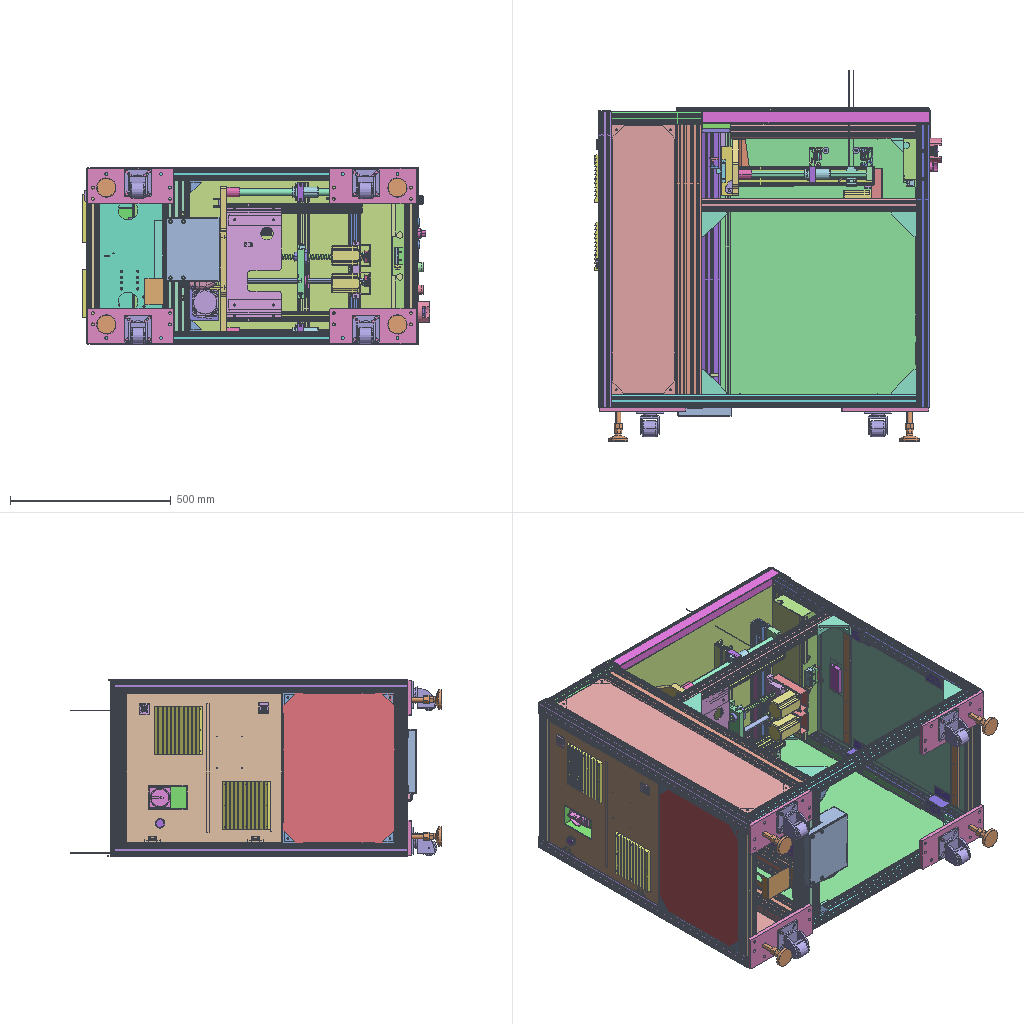Assembly | STEP file | 138 different items | 315 placed | box 1081 x 1155 x 550 mm
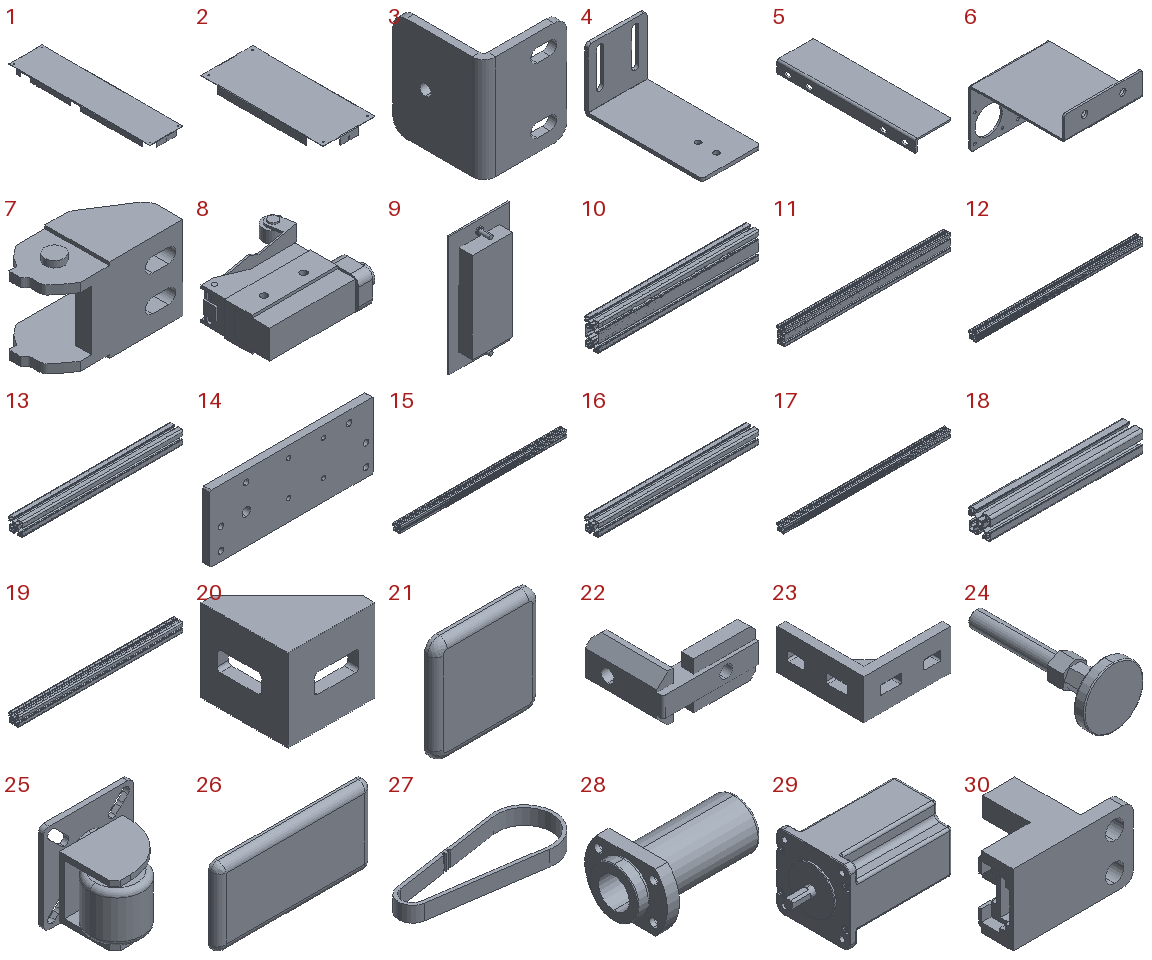Parts list (item | name | quantity | parent item | size | volume):
1 | - | x2 | - | 199 x 839 x 30 mm | 251918 mm3
2 | - | x1 | - | 199 x 469 x 30 mm | 138914 mm3
3 | - | x4 | - | 32 x 35 x 40 mm | 7142 mm3
4 | - | x1 | - | 35 x 70 x 37 mm | 6884 mm3
5 | - | x1 | - | 68 x 260 x 23 mm | 66736 mm3
6 | - | x1 | - | 82 x 100 x 83 mm | 26763 mm3
7 | Cable carrier connector 15x20B | x2 | - | 40 x 20 x 28 mm | 6776 mm3
8 | Limit switch D4MC-2000 | x1 | - | 71.855 x 71.5 x 21.7 mm | 42318 mm3
9 | Concealed handle XAD01_304_Yihe Da | x1 | - | 60 x 15 x 119 mm | 18675 mm3
10 | - | x2 | - | 470 x 40 x 80 mm | 377061 mm3
11 | - | x4 | - | 840 x 40 x 80 mm | 681890 mm3
12 | - | x2 | - | 880 x 40 x 40 mm | 420476 mm3
13 | - | x1 | - | 470 x 40 x 40 mm | 224394 mm3
14 | - | x4 | - | 270 x 12 x 110 mm | 348133 mm3
15 | MK-8-4040C-L-00 profile 4040C standard 950mm | x2 | - | 950 x 40 x 40 mm | 454336 mm3
16 | MK-8-4040C-L-00 profile 4040C standard 470mm | x3 | - | 470 x 40 x 40 mm | 224777 mm3
17 | MK-8-4040C-L-00 profile 4040C standard 920mm | x2 | - | 920 x 40 x 40 mm | 439989 mm3
18 | MK-8-4040C-L-00 profile 4040C standard 280mm | x2 | - | 280 x 40 x 40 mm | 133910 mm3
19 | MK-8-4040C-L-00 profile 4040C standard 670mm | x2 | - | 670 x 40 x 40 mm | 320427 mm3
20 | Die-cast aluminium connector, 40 series, 40mm face, standard type | x32 | - | 38 x 38 x 36 mm | 14409 mm3
21 | End cap panel MK-EC-B-4040x4.2 | x6 | - | 40 x 12.4 x 40 mm | 5038 mm3
22 | New in-slot right-angle connector, 40 series (with set screw) | x6 | - | 38 x 31 x 18.5 mm | 6406 mm3
23 | Die-cast aluminium connector, 40 series, 40mm face, reinforced type | x8 | - | 78 x 78 x 36 mm | 52626 mm3
24 | All-carbon-steel swivel leveling foot KCUF M16-100-60-electrophoretic black | x4 | - | 60 x 139 x 60 mm | 70730 mm3
25 | Medium 2-inch swivel caster J38NZN050R | x4 | - | 90 x 79 x 85 mm | 121466 mm3
26 | End cap panel MK-EC-B-3060x4 | x2 | - | 60 x 12.2 x 30 mm | 5483 mm3
27 | Timing belt 210-3M-9mm wide_16-36 | x2 | - | 90.97 x 35.218 x 9 mm | 3580 mm3
28 | Guided double-liner flanged linear bearing LML21-d20 | x2 | - | 80 x 54 x 38 mm | 45928 mm3
29 | Stepper motor SS2403A42A | x2 | - | 105.6 x 60 x 60 mm | 258866 mm3
30 | Photoelectric sensor PM-Y65 | x1 | - | 22.7 x 14.9 x 13.4 mm | 1660 mm3
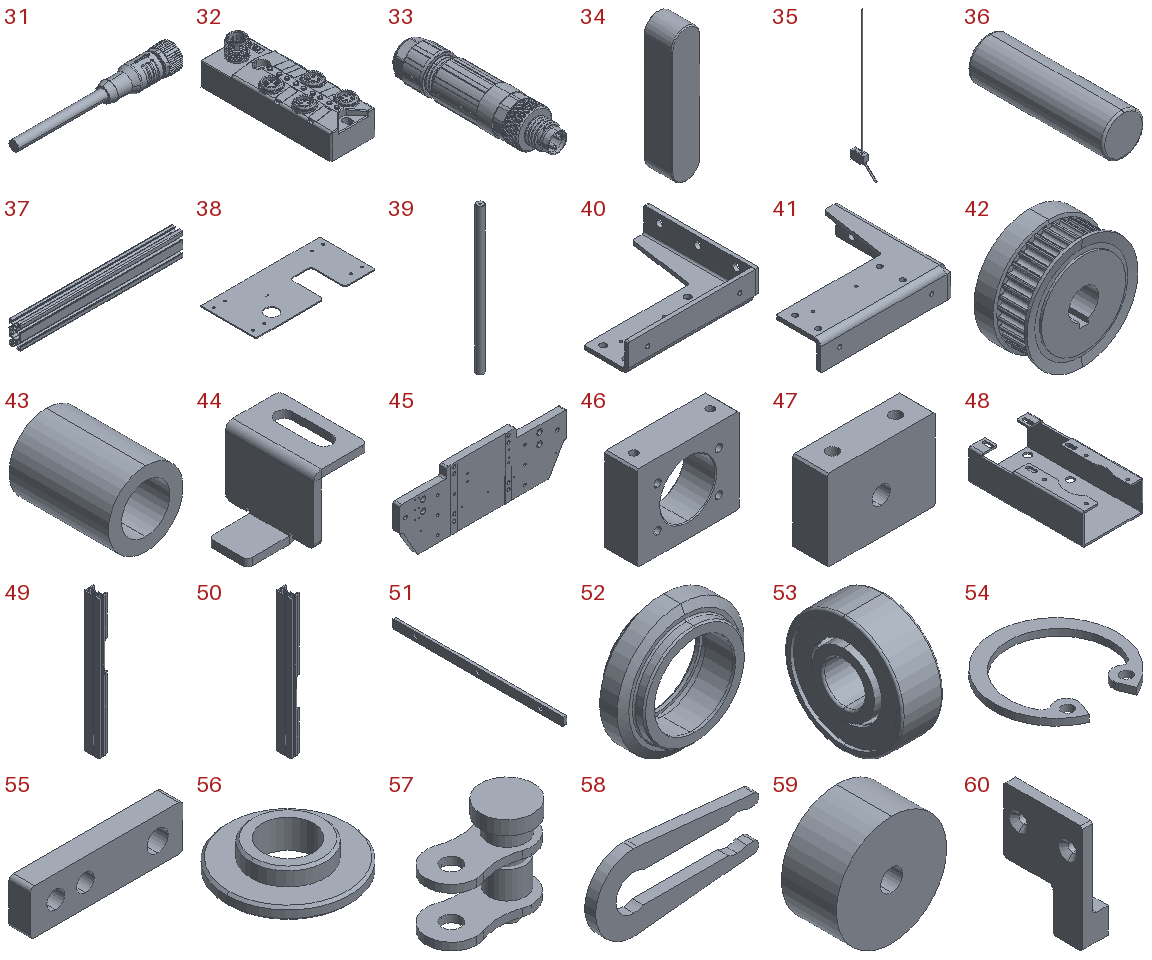31 | - | x1 | - | 99 x 14.979 x 14.996 mm | 5984 mm3
32 | I/O junction box 23N4S1 | x1 | - | 29.939 x 86.939 x 25.75 mm | 38975 mm3
33 | Plug (straight male) | x4 | - | - | -
34 | Type A plain key 3x3x14 | x2 | - | 3 x 3 x 14 mm | 119.894 mm3
35 | Miniature photoelectric sensor CX-442 | x2 | - | 11.2 x 58.715 x 345.215 mm | 7993 mm3
36 | - | x2 | - | 6 x 19.5 x 6 mm | 550.638 mm3
37 | - | x2 | - | 417 x 30 x 60.001 mm | 241330 mm3
38 | - | x1 | - | 365 x 170 x 3 mm | 161069 mm3
39 | - | x2 | - | 20 x 20 x 410 mm | 128595 mm3
40 | - | x1 | - | 170 x 145 x 37 mm | 104270 mm3
41 | - | x1 | - | 170 x 145 x 37 mm | 104662 mm3
42 | - | x2 | - | 37 x 19 x 37 mm | 15386 mm3
43 | - | x2 | - | 30 x 40 x 30 mm | 16328 mm3
44 | - | x1 | - | 19.5 x 18 x 15 mm | 668.205 mm3
45 | - | x1 | - | 482 x 20 x 176 mm | 1391575 mm3
46 | - | x2 | - | 60 x 19 x 50 mm | 36440 mm3
47 | - | x2 | - | 60 x 19 x 45 mm | 39956 mm3
48 | - | x2 | - | 68 x 128 x 35 mm | 37554 mm3
49 | - | x1 | - | 35 x 55 x 500 mm | 378713 mm3
50 | - | x1 | - | 35 x 55 x 500 mm | 378713 mm3
51 | - | x2 | - | 9 x 410 x 20.4 mm | 65356 mm3
52 | - | x4 | - | 25 x 8.5 x 25 mm | 1521 mm3
53 | PN_0001 Deep groove ball bearing 606-ZZ | x8 | - | 6 x 17 x 17 mm | 776.566 mm3
54 | PN_0001 Bore retaining ring type A 17 | x8 | - | 18.3 x 17.603 x 1 mm | 85.781 mm3
55 | - | x4 | - | 36 x 5 x 10.6 mm | 1667 mm3
56 | - | x4 | - | 15 x 15 x 3.5 mm | 281.21 mm3
57 | 06B side guide wheel chain | x2 | - | 18.325 x 9 x 17.4 mm | 854.513 mm3
58 | 06B side guide wheel chain link | x2 | - | 15 x 1 x 7 mm | 49.292 mm3
59 | - | x2 | - | 20 x 10 x 20 mm | 2790 mm3
60 | - | x1 | - | 13 x 40 x 55 mm | 9570 mm3
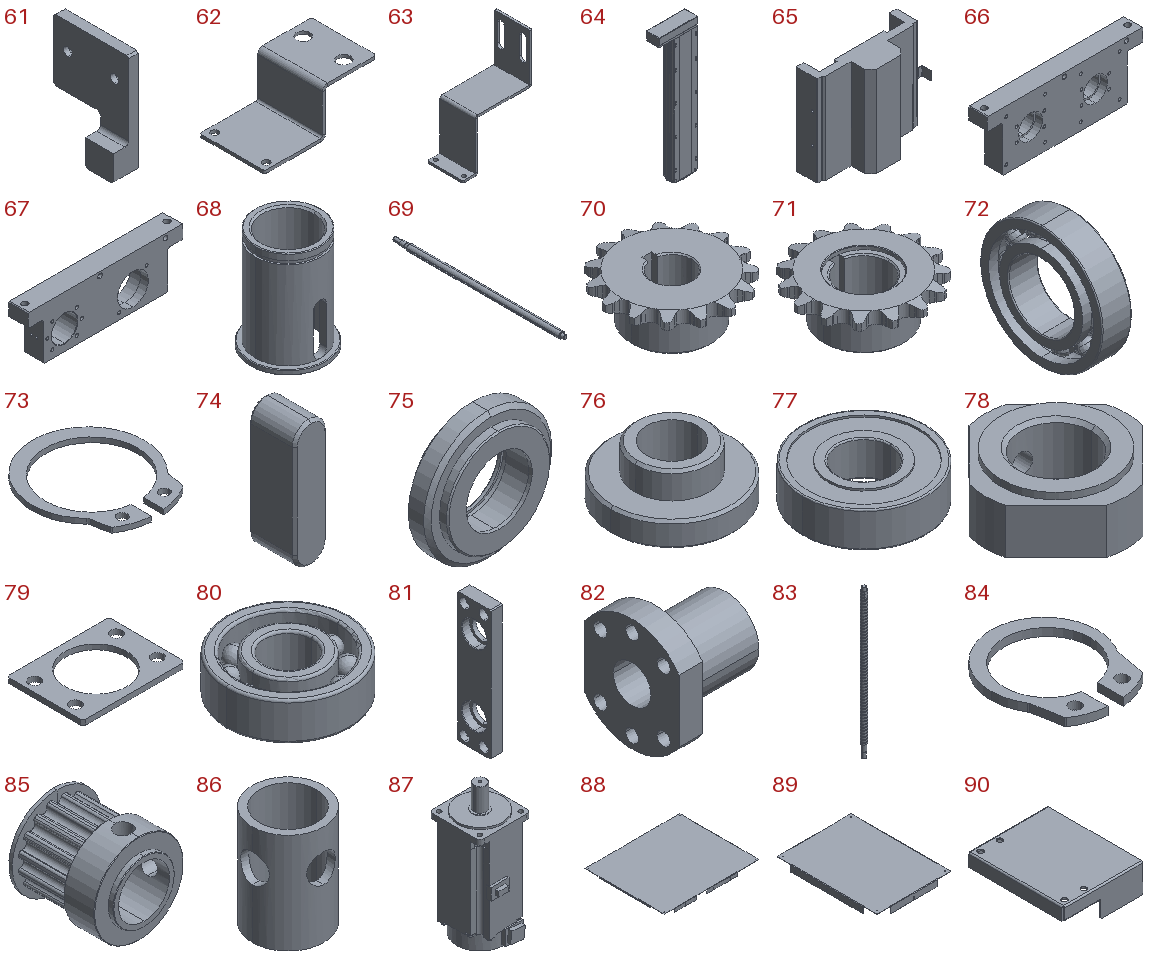61 | - | x1 | - | 13 x 40 x 55 mm | 9570 mm3
62 | - | x1 | - | 55 x 32 x 23.5 mm | 3494 mm3
63 | - | x1 | - | 62 x 32 x 90 mm | 8899 mm3
64 | Single-axis manipulator CFS17-L10-650-BR-T750-C4-MB-3M-body | x1 | - | 280.5 x 91 x 933.5 mm | 7444540 mm3
65 | Single-axis manipulator CFS17-L10-650-BR-T750-C4-MB-3M-slider | x1 | - | 177 x 71 x 152 mm | 741184 mm3
66 | - | x1 | - | 180 x 21 x 68 mm | 190682 mm3
67 | - | x1 | - | 170 x 21 x 57 mm | 135678 mm3
68 | - | x1 | - | 23 x 23 x 31.4 mm | 3535 mm3
69 | - | x1 | - | 16 x 443 x 16 mm | 80862 mm3
70 | - | x1 | - | 50.395 x 50.132 x 19 mm | 15455 mm3
71 | - | x1 | - | 50.395 x 50.132 x 19.5 mm | 13040 mm3
72 | Bearing 6904Z | x1 | - | 9 x 37 x 37 mm | 4601 mm3
73 | Shaft retaining ring type A 20 | x1 | - | 22.5 x 25.161 x 1 mm | 155.824 mm3
74 | - | x1 | - | 3.9 x 5.5 x 15 mm | 300.753 mm3
75 | - | x4 | - | 31 x 9 x 31 mm | 3611 mm3
76 | - | x4 | - | 15 x 15 x 6.2 mm | 541.108 mm3
77 | Bearing 6001ZZ | x2 | - | 28 x 28 x 8 mm | 3776 mm3
78 | - | x1 | - | 22 x 22 x 8 mm | 1773 mm3
79 | - | x2 | - | 40 x 30 x 2 mm | 1364 mm3
80 | Bearing 6000Z_P5_BONA_eco-friendly | x2 | - | 26 x 26 x 8 mm | 2544 mm3
81 | - | x1 | - | 12 x 35 x 135 mm | 43258 mm3
82 | Nut SFU01604-4 | x1 | in Ball screw assembly SFUR01604T4DFC7-445-P0 | 40 x 40 x 48 mm | 25660 mm3
83 | Ball screw assembly SFUR1604-445 | x1 | in Ball screw assembly SFUR01604T4DFC7-445-P0 | 16 x 16 x 445 mm | 80049 mm3
84 | Shaft retaining ring type A 12 | x1 | - | 13.6 x 15.973 x 1 mm | 68.14 mm3
85 | - | x2 | - | 17.5 x 18 x 17.5 mm | 1873 mm3
86 | - | x2 | - | 10 x 10 x 14 mm | 370.028 mm3
87 | Servo motor HG-KN73BJK-S100 750w_with brake_with keyway_Mitsubishi | x1 | - | 80.44 x 89.02 x 202.7 mm | 918886 mm3
88 | - | x1 | - | 798 x 668 x 30 mm | 686782 mm3
89 | - | x1 | - | 349 x 469 x 30 mm | 233516 mm3
90 | - | x1 | - | 166 x 200 x 60 mm | 160354 mm3
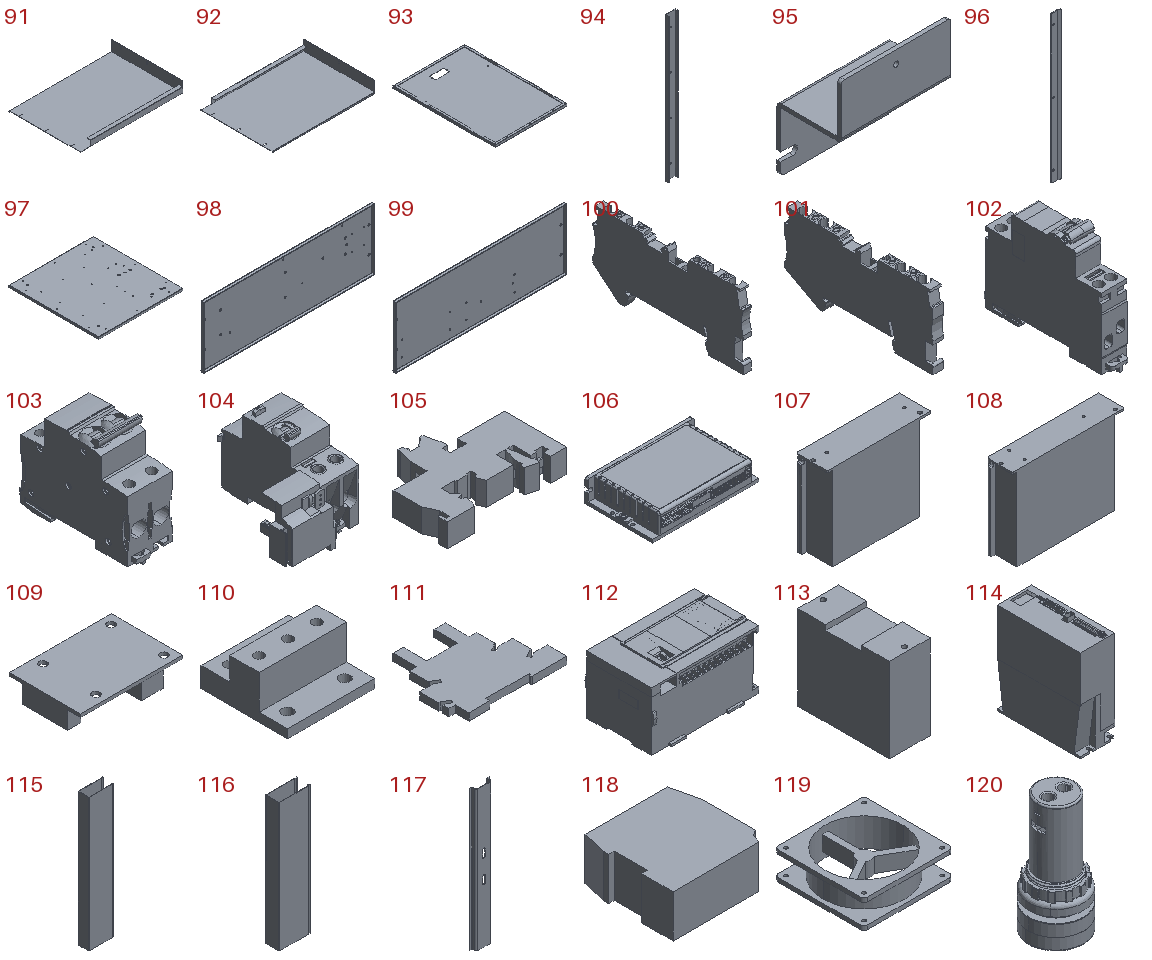91 | - | x1 | - | 790 x 550 x 88 mm | 1058095 mm3
92 | - | x1 | - | 790 x 550 x 88 mm | 1059109 mm3
93 | - | x1 | - | 467 x 667 x 16 mm | 433959 mm3
94 | - | x2 | - | 30 x 10 x 440 mm | 30430 mm3
95 | - | x4 | - | 70 x 41 x 71.5 mm | 18730 mm3
96 | - | x1 | - | 22.338 x 5 x 350 mm | 15718 mm3
97 | - | x1 | - | 400 x 425 x 10 mm | 275109 mm3
98 | - | x1 | - | 398 x 7.5 x 143 mm | 93935 mm3
99 | - | x1 | - | 398 x 7.5 x 143 mm | 94056 mm3
100 | Feed-through terminal block PT 1.5-S-QUATTRO | x27 | - | 3.5 x 63.2 x 30.5 mm | 4808 mm3
101 | Feed-through terminal block PT2,5-QUATTRO-3209578 | x6 | - | 5.15 x 72.2 x 35.25 mm | 9561 mm3
102 | Schneider miniature circuit breaker iDPNN-1P+N-C10A | x1 | - | 17.5 x 90.6 x 73.848 mm | 76092 mm3
103 | Miniature circuit breaker IC65N-2P-C16A | x1 | - | 35.4 x 93.9 x 74.3 mm | 159125 mm3
104 | Residual current device Vigi-iC65-ELE-2P-40A-30mA-A | x1 | - | 76.2 x 105.618 x 73.908 mm | 172404 mm3
105 | End bracket-E UK-1201442 | x4 | - | 50.5 x 35.3 x 9.5 mm | 9735 mm3
106 | Stepper motor driver DM542-KK V3.0 | x2 | - | 119 x 77.6 x 25.5 mm | 99944 mm3
107 | Switching power supply LRS-50-24 (Mean Well) | x1 | - | 99 x 30 x 82 mm | 213867 mm3
108 | Switching power supply LRS-100-48 | x1 | - | 129 x 30 x 97 mm | 340596 mm3
109 | PCB assembly | x1 | - | 54 x 38 x 11.5 mm | 8666 mm3
110 | Six-position earth copper block | x2 | - | 30.3 x 30.2 x 15 mm | 7115 mm3
111 | Ultra-miniature medium-power relay HF41F_24-ZST and socket 41F-1Z-C2-1 | x1 | - | 88 x 75.5 x 6.1 mm | 25363 mm3
112 | PLC module FX5U-32MT_ES | x1 | - | 150 x 96.4 x 84.9 mm | 980252 mm3
113 | PLC expansion IO FX5-16ET_ES8 (inputs, 8 outputs, transistor sink type) | x1 | - | 40 x 90 x 83 mm | 291482 mm3
114 | Servo drive MR-JE-70A | x1 | - | 70 x 168 x 191.95 mm | 896378 mm3
115 | Cable trough 35_L430 | x2 | - | 80.625 x 35 x 430 mm | 84214 mm3
116 | Cable trough 35_L330 | x3 | - | 80.625 x 35 x 330 mm | 64629 mm3
117 | Guide rail L_L245 | x2 | - | 35 x 8.3 x 245 mm | 11487 mm3
118 | EMC filter FIL-1S-1-10A-230AC-UT   1292320 | x1 | - | 99.5 x 99 x 45 mm | 422145 mm3
119 | Axial fan 1238A2MBL | x1 | - | 120 x 120 x 38 mm | 111801 mm3
120 | Indicator light AD17-22-AC220VW white | x1 | - | 29 x 29.009 x 63.018 mm | 9405 mm3
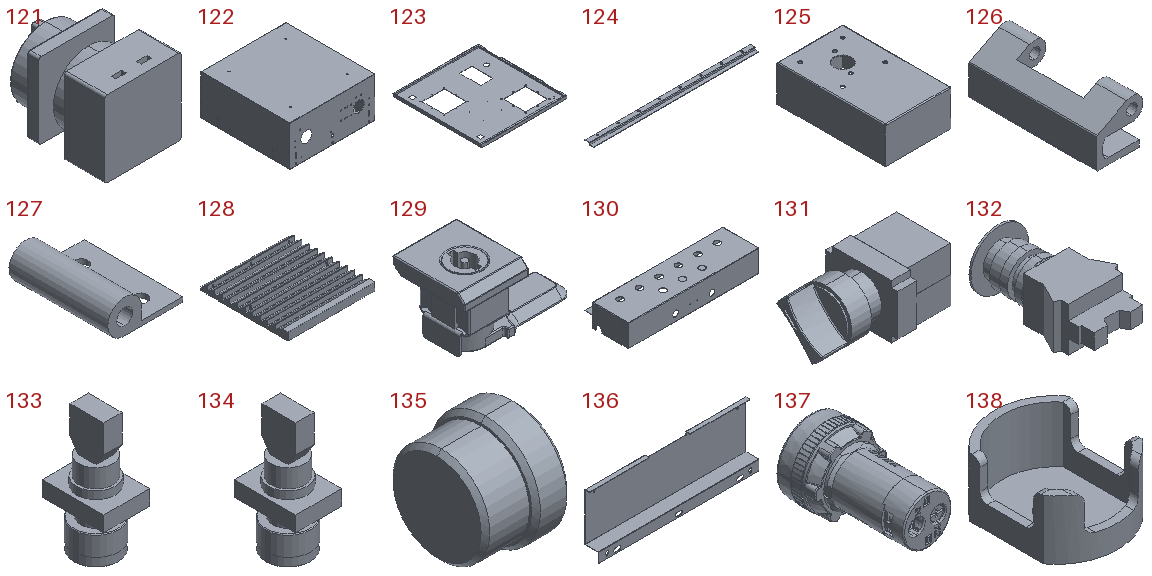121 | Power switch LW42B2-1824_L | x1 | - | 65.5 x 92 x 65.5 mm | 250369 mm3
122 | - | x1 | - | 465 x 486 x 234 mm | 846762 mm3
123 | - | x1 | - | 465 x 484 x 17 mm | 267277 mm3
124 | - | x1 | - | 400 x 21 x 6 mm | 10098 mm3
125 | - | x1 | - | 74 x 122 x 41 mm | 24069 mm3
126 | Hinge CL237Z3H001-01 | x2 | in Hinge CL237Z3H001 | 17.5 x 48 x 18 mm | 5234 mm3
127 | Hinge CL237Z3H001-02 | x2 | in Hinge CL237Z3H001 | 19 x 25 x 8.5 mm | 1495 mm3
128 | Class B ventilation filter assembly ZL-803 (7032 adhesive) | x2 | - | 150 x 150 x 28 mm | 421271 mm3
129 | Cylinder lock MS813-Shengjiu | x2 | - | 58.793 x 35 x 31.6 mm | 16415 mm3
130 | - | x1 | - | 469 x 158.8 x 80 mm | 180608 mm3
131 | Short-handle selector switch XB2-BD21C | x1 | - | 70 x 40 x 30 mm | 44517 mm3
132 | - | x1 | - | 44.567 x 87.5 x 40 mm | 63672 mm3
133 | Green illuminated pushbutton XB2-BW33B1C with 1 NO contact | x1 | - | 30 x 40 x 80 mm | 40739 mm3
134 | Blue illuminated pushbutton XB2-BW36B1C with 1 NO contact | x1 | - | 30 x 40 x 80 mm | 40739 mm3
135 | Panel plug T02 | x2 | - | 18 x 25 x 25 mm | 7618 mm3
136 | - | x1 | - | 470 x 39.5 x 167.8 mm | 118270 mm3
137 | Buzzer XB2BSB4LC | x1 | - | 29.699 x 50.596 x 29.699 mm | 12548 mm3
138 | - | x1 | - | 64 x 80 x 38.5 mm | 37425 mm3
Placements (level | parent | child | x y z in mm | rotation matrix by rows), first 274 of 336 lines:
1 | subassembly 2 | subassembly 3 | 777.434 1281.272 1459.066 | -1 0 0 0 1 0 0 0 -1
1 | subassembly 2 | subassembly 3 | 777.434 1281.272 2007.466 | 1 0 0 0 1 0 0 0 1
1 | subassembly 2 | subassembly 4 | 777.434 1740.472 1733.266 | 1 0 0 0 0 1 0 -1 0
1 | subassembly 2 | subassembly 5 | 677.434 1605.272 1965.766 | 0 1 0 0 0 1 1 0 -0
1 | subassembly 2 | subassembly 5 | 677.434 1605.272 1500.766 | 0 1 0 0 0 -1 -1 0 0
1 | subassembly 2 | subassembly 6 | 922.434 1263.772 1878.266 | 0 0 1 -1 0 0 0 -1 0
1 | subassembly 2 | subassembly 7 | 914.434 1189.272 1583.266 | -1 0 0 0 0 1 0 1 -0
1 | subassembly 2 | subassembly 5 | 677.434 1305.272 1965.766 | 0 1 0 0 0 1 1 0 -0
1 | subassembly 2 | subassembly 5 | 677.434 1305.272 1500.766 | 0 1 0 0 0 -1 -1 0 0
1 | subassembly 2 | subassembly 8 | 817.434 941.272 1623.266 | 0 -1 0 0 0 -1 1 0 -0
1 | subassembly 2 | Cable carrier connector 15x20B | 922.434 1230.772 1911.766 | 0 1 0 1 0 0 0 0 -1
1 | subassembly 2 | Cable carrier connector 15x20B | 1054.434 1486.772 1885.766 | 0 -1 0 1 0 0 0 0 1
1 | subassembly 2 | Limit switch D4MC-2000 | 1615.435 1519.422 1745.966 | 0 1 0 0 0 -1 -1 0 0
1 | subassembly 2 | Concealed handle XAD01_304_Yihe Da | 1654.034 1457.272 1733.266 | 0 1 0 -1 0 0 0 0 1
1 | subassembly 2 | subassembly 9 | 817.116 381.543 740.825 | 1 0 0 0 1 0 0 0 1
2 | subassembly 9 | subassembly 10 | 100.319 459.73 1227.441 | 0 0 1 0 1 0 -1 0 0
2 | subassembly 9 | subassembly 10 | 100.319 1339.73 757.441 | 0 0 1 0 -1 0 1 0 0
2 | subassembly 9 | subassembly 11 | 120.319 479.73 1062.441 | 0 -1 0 1 0 0 0 0 1
2 | subassembly 9 | subassembly 11 | 120.319 479.73 882.441 | 0 -1 0 1 0 0 0 0 1
2 | subassembly 9 | subassembly 11 | 100.319 479.73 737.441 | 0 0 1 1 0 0 0 1 -0
2 | subassembly 9 | subassembly 11 | 100.319 479.73 1247.441 | 0 0 1 1 0 0 0 1 -0
2 | subassembly 9 | subassembly 12 | 830.319 1319.73 1247.441 | 0 0 -1 -1 0 0 0 1 0
2 | subassembly 9 | subassembly 13 | 830.319 1299.73 757.441 | 0 0 -1 0 1 0 1 0 0
2 | subassembly 9 | subassembly 12 | 830.319 1319.73 737.441 | 0 0 1 -1 0 0 0 -1 0
2 | subassembly 9 | subassembly 14 | -177.681 433.73 719.441 | 1 0 0 0 -1 0 0 0 -1
2 | subassembly 9 | subassembly 14 | -177.681 433.73 1265.441 | 1 0 0 0 1 0 0 0 1
2 | subassembly 9 | subassembly 14 | 848.319 433.73 1265.441 | -1 0 0 0 -1 0 0 0 1
2 | subassembly 9 | subassembly 14 | 848.319 433.73 719.441 | -1 0 0 0 1 0 0 0 -1
2 | subassembly 9 | MK-8-4040C-L-00 profile 4040C standard 950mm | -139.681 459.73 737.441 | 1 0 0 0 1 0 0 0 1
2 | subassembly 9 | MK-8-4040C-L-00 profile 4040C standard 950mm | -139.681 459.73 1247.441 | 1 0 0 0 1 0 0 0 1
2 | subassembly 9 | MK-8-4040C-L-00 profile 4040C standard 470mm | -159.681 459.73 757.441 | 0 0 -1 0 1 0 1 0 0
2 | subassembly 9 | MK-8-4040C-L-00 profile 4040C standard 470mm | 830.319 459.73 757.441 | 0 0 -1 0 1 0 1 0 0
2 | subassembly 9 | MK-8-4040C-L-00 profile 4040C standard 470mm | -159.681 1339.73 757.441 | 0 0 -1 0 1 0 1 0 0
2 | subassembly 9 | MK-8-4040C-L-00 profile 4040C standard 920mm | -159.681 439.73 1247.441 | 0 -1 0 1 0 0 0 0 1
2 | subassembly 9 | MK-8-4040C-L-00 profile 4040C standard 920mm | -159.681 439.73 737.441 | 0 -1 0 1 0 0 0 0 1
2 | subassembly 9 | MK-8-4040C-L-00 profile 4040C standard 280mm | -139.681 1339.73 1247.441 | 1 0 0 0 1 0 0 0 1
2 | subassembly 9 | MK-8-4040C-L-00 profile 4040C standard 280mm | -139.681 1339.73 737.441 | 1 0 0 0 1 0 0 0 1
2 | subassembly 9 | MK-8-4040C-L-00 profile 4040C standard 670mm | 140.319 1299.73 737.441 | 1 0 0 0 1 0 0 0 1
2 | subassembly 9 | MK-8-4040C-L-00 profile 4040C standard 670mm | 140.319 1069.73 1247.441 | 1 0 0 0 1 0 0 0 1
2 | subassembly 9 | Die-cast aluminium connector, 40 series, 40mm face, standard type | -139.681 479.73 737.441 | 1 0 0 0 1 0 0 0 1
2 | subassembly 9 | Die-cast aluminium connector, 40 series, 40mm face, standard type | -139.681 1319.73 737.441 | 0 1 0 -1 0 0 0 0 1
2 | subassembly 9 | Die-cast aluminium connector, 40 series, 40mm face, standard type | 60.319 479.73 737.291 | 0 -1 0 1 0 0 0 0 1
2 | subassembly 9 | Die-cast aluminium connector, 40 series, 40mm face, standard type | 60.319 1319.73 737.441 | -1 0 0 0 -1 0 0 0 1
2 | subassembly 9 | Die-cast aluminium connector, 40 series, 40mm face, standard type | -139.681 1319.73 1247.441 | 1 0 0 0 -1 0 0 0 -1
2 | subassembly 9 | Die-cast aluminium connector, 40 series, 40mm face, standard type | -139.681 479.73 1247.441 | 0 1 0 1 0 0 0 0 -1
2 | subassembly 9 | Die-cast aluminium connector, 40 series, 40mm face, standard type | 60.319 479.73 1247.441 | -1 0 0 0 1 0 0 0 -1
2 | subassembly 9 | Die-cast aluminium connector, 40 series, 40mm face, standard type | 60.319 1319.73 1247.441 | 0 -1 0 -1 0 0 0 0 -1
2 | subassembly 9 | Die-cast aluminium connector, 40 series, 40mm face, standard type | 60.319 1339.73 1227.441 | -1 0 0 0 0 -1 0 -1 -0
2 | subassembly 9 | Die-cast aluminium connector, 40 series, 40mm face, standard type | 60.319 1339.73 757.441 | 0 -1 0 0 0 -1 1 0 -0
2 | subassembly 9 | Die-cast aluminium connector, 40 series, 40mm face, standard type | -139.681 1339.73 757.441 | 1 0 0 0 0 -1 0 1 0
2 | subassembly 9 | Die-cast aluminium connector, 40 series, 40mm face, standard type | 60.319 459.73 1227.441 | -1 0 0 0 0 -1 0 -1 -0
2 | subassembly 9 | Die-cast aluminium connector, 40 series, 40mm face, standard type | 60.319 459.73 757.441 | 0 -1 0 0 0 -1 1 0 0
2 | subassembly 9 | Die-cast aluminium connector, 40 series, 40mm face, standard type | 140.319 459.73 1227.441 | 0 1 0 0 0 -1 -1 0 0
2 | subassembly 9 | Die-cast aluminium connector, 40 series, 40mm face, standard type | 80.169 1319.73 1227.441 | 0 0 -1 0 -1 0 -1 0 0
2 | subassembly 9 | Die-cast aluminium connector, 40 series, 40mm face, standard type | 80.169 1319.73 757.441 | 0 0 -1 -1 0 0 0 1 -0
2 | subassembly 9 | Die-cast aluminium connector, 40 series, 40mm face, standard type | -139.681 1339.73 1227.441 | 0 1 0 0 0 -1 -1 0 0
2 | subassembly 9 | Die-cast aluminium connector, 40 series, 40mm face, standard type | 140.319 459.73 757.441 | 1 0 0 0 0 -1 0 1 0
2 | subassembly 9 | End cap panel MK-EC-B-4040x4.2 | -159.681 1363.93 737.441 | -1 0 0 0 -1 0 0 0 1
2 | subassembly 9 | End cap panel MK-EC-B-4040x4.2 | -159.681 1363.93 1247.441 | -1 0 0 0 -1 0 0 0 1
2 | subassembly 9 | New in-slot right-angle connector, 40 series (with set screw) | 834.319 1290.73 1238.341 | 0 0 -1 0 -1 0 -1 0 0
2 | subassembly 9 | New in-slot right-angle connector, 40 series (with set screw) | 826.319 1290.73 746.541 | 0 0 1 0 -1 0 1 0 -0
2 | subassembly 9 | Die-cast aluminium connector, 40 series, 40mm face, standard type | 122.319 479.73 1227.441 | 0 0 -1 1 0 0 0 -1 0
2 | subassembly 9 | Die-cast aluminium connector, 40 series, 40mm face, standard type | 78.319 479.73 1227.441 | 0 0 -1 1 0 0 0 -1 0
2 | subassembly 9 | Die-cast aluminium connector, 40 series, 40mm face, standard type | 122.319 1319.73 1227.441 | 0 0 -1 0 -1 0 -1 0 0
2 | subassembly 9 | Die-cast aluminium connector, 40 series, 40mm face, standard type | 122.319 1319.73 757.441 | 0 0 -1 -1 0 0 0 1 -0
2 | subassembly 9 | Die-cast aluminium connector, 40 series, 40mm face, standard type | 100.319 479.73 860.441 | -1 0 0 0 1 0 0 0 -1
2 | subassembly 9 | Die-cast aluminium connector, 40 series, 40mm face, standard type | 100.319 479.73 1084.441 | -1 0 0 0 1 0 0 0 -1
2 | subassembly 9 | Die-cast aluminium connector, 40 series, 40mm face, standard type | 100.319 1319.73 1084.441 | 0 -1 0 -1 0 0 0 0 -1
2 | subassembly 9 | Die-cast aluminium connector, 40 series, 40mm face, standard type | 100.319 1319.73 860.441 | 0 -1 0 -1 0 0 0 0 -1
2 | subassembly 9 | Die-cast aluminium connector, 40 series, 40mm face, standard type | -161.681 479.73 1227.441 | 0 0 -1 1 0 0 0 -1 0
2 | subassembly 9 | Die-cast aluminium connector, 40 series, 40mm face, standard type | -161.681 479.73 757.441 | 0 0 1 1 0 0 0 1 -0
2 | subassembly 9 | New in-slot right-angle connector, 40 series (with set screw) | 826.419 465.73 1241.441 | 0 0 1 0 1 0 -1 0 -0
2 | subassembly 9 | New in-slot right-angle connector, 40 series (with set screw) | 834.219 465.73 743.441 | 0 0 -1 0 1 0 1 0 0
2 | subassembly 9 | New in-slot right-angle connector, 40 series (with set screw) | -155.781 1333.73 743.441 | 0 0 -1 -1 0 0 0 1 0
2 | subassembly 9 | New in-slot right-angle connector, 40 series (with set screw) | -163.581 1333.73 1241.441 | 0 0 1 -1 0 0 0 -1 -0
2 | subassembly 9 | Die-cast aluminium connector, 40 series, 40mm face, standard type | -161.681 829.73 757.441 | 0 0 -1 -1 0 0 0 1 -0
2 | subassembly 9 | Die-cast aluminium connector, 40 series, 40mm face, standard type | -161.681 829.73 1227.441 | 0 0 1 -1 0 0 0 -1 -0
2 | subassembly 9 | Die-cast aluminium connector, 40 series, 40mm face, reinforced type | 140.319 479.73 719.441 | 1 0 0 0 1 0 0 0 1
2 | subassembly 9 | Die-cast aluminium connector, 40 series, 40mm face, reinforced type | 140.319 479.73 1265.441 | 0 1 0 1 0 0 0 0 -1
2 | subassembly 9 | Die-cast aluminium connector, 40 series, 40mm face, reinforced type | 140.319 1049.73 1265.441 | 1 0 0 0 -1 0 0 0 -1
2 | subassembly 9 | Die-cast aluminium connector, 40 series, 40mm face, reinforced type | 140.319 1279.73 719.441 | 0 1 0 -1 0 0 0 0 1
2 | subassembly 9 | Die-cast aluminium connector, 40 series, 40mm face, reinforced type | 810.319 479.73 1265.441 | -1 0 0 0 1 0 0 0 -1
2 | subassembly 9 | Die-cast aluminium connector, 40 series, 40mm face, reinforced type | 810.319 479.73 719.441 | 0 -1 0 1 0 0 0 0 1
2 | subassembly 9 | Die-cast aluminium connector, 40 series, 40mm face, reinforced type | 810.319 1279.73 719.441 | -1 0 0 0 -1 0 0 0 1
2 | subassembly 9 | Die-cast aluminium connector, 40 series, 40mm face, reinforced type | 810.319 1049.73 1265.441 | 0 -1 0 -1 0 0 0 0 -1
2 | subassembly 9 | End cap panel MK-EC-B-4040x4.2 | 830.319 1323.93 1247.441 | -1 0 0 0 -1 0 0 0 1
2 | subassembly 9 | End cap panel MK-EC-B-4040x4.2 | 830.319 1323.93 737.441 | -1 0 0 0 -1 0 0 0 1
2 | subassembly 9 | End cap panel MK-EC-B-4040x4.2 | 144.519 1339.73 1247.441 | 0 -1 0 1 0 0 0 0 1
2 | subassembly 9 | End cap panel MK-EC-B-4040x4.2 | 144.519 1339.73 737.441 | 0 -1 0 1 0 0 0 0 1
2 | subassembly 9 | Die-cast aluminium connector, 40 series, 40mm face, standard type | 78.319 479.73 757.441 | 0 0 1 1 0 0 0 1 -0
2 | subassembly 9 | Die-cast aluminium connector, 40 series, 40mm face, standard type | 122.319 479.73 757.441 | 0 0 -1 0 1 0 1 0 -0
2 | subassembly 9 | All-carbon-steel swivel leveling foot KCUF M16-100-60-electrophoretic black | -117.681 334.73 1205.441 | 0.6837 0 -0.7298 0 1 0 0.7298 0 0.6837
2 | subassembly 9 | All-carbon-steel swivel leveling foot KCUF M16-100-60-electrophoretic black | -117.681 334.73 779.441 | 0.6837 0 -0.7298 0 1 0 0.7298 0 0.6837
2 | subassembly 9 | All-carbon-steel swivel leveling foot KCUF M16-100-60-electrophoretic black | 788.319 334.73 779.441 | 0.6837 0 -0.7298 0 1 0 0.7298 0 0.6837
2 | subassembly 9 | All-carbon-steel swivel leveling foot KCUF M16-100-60-electrophoretic black | 788.319 334.73 1205.441 | 0.6837 0 -0.7298 0 1 0 0.7298 0 0.6837
2 | subassembly 9 | Medium 2-inch swivel caster J38NZN050R | -20.104 422.73 1219.864 | 0 0 -1 0 1 0 1 0 0
2 | subassembly 9 | Medium 2-inch swivel caster J38NZN050R | 689.504 422.73 1218.627 | 0 0 -1 0 1 0 1 0 0
2 | subassembly 9 | Medium 2-inch swivel caster J38NZN050R | -18.866 422.73 766.256 | 0 0 -1 0 1 0 1 0 0
2 | subassembly 9 | Medium 2-inch swivel caster J38NZN050R | 689.504 422.73 766.256 | 0 0 -1 0 1 0 1 0 0
1 | subassembly 2 | subassembly 15 | 804.051 1822.324 1868.016 | 1 0 0 0 1 0 0 0 1
2 | subassembly 15 | End cap panel MK-EC-B-3060x4 | 691.383 -280.052 12.751 | 0 -1 0 1 0 0 0 0 1
2 | subassembly 15 | End cap panel MK-EC-B-3060x4 | 691.383 -280.052 -322.25 | 0 -1 0 1 0 0 0 0 1
2 | subassembly 15 | Timing belt 210-3M-9mm wide_16-36 | 695.883 -353.982 -219.179 | 0 0 1 0.9944 -0.1061 0 0.1061 0.9944 -0
2 | subassembly 15 | Timing belt 210-3M-9mm wide_16-36 | 695.883 -353.982 -133.32 | 0 0 1 0.9982 0.06018 0 -0.06018 0.9982 0
2 | subassembly 15 | Guided double-liner flanged linear bearing LML21-d20 | 474.761 -275.052 64.251 | 1 0 0 0 0 -1 0 1 -0
2 | subassembly 15 | Guided double-liner flanged linear bearing LML21-d20 | 474.761 -275.052 -373.75 | 1 0 0 0 0 1 0 -1 0
2 | subassembly 15 | Stepper motor SS2403A42A | 682.544 -353.982 -219.179 | -1 0 0 0 1 0 0 0 -1
2 | subassembly 15 | Stepper motor SS2403A42A | 682.544 -353.982 -133.32 | -1 0 0 0 1 0 0 0 -1
2 | subassembly 15 | Photoelectric sensor PM-Y65 | 338.383 -297.152 -102.749 | 1 0 0 0 1 0 0 0 1
2 | subassembly 15 | subassembly 16 | 339.983 -272.068 -60.213 | 0 0.3525 0.9358 0 -0.9358 0.3525 1 0 0
2 | subassembly 15 | I/O junction box 23N4S1 | 405.833 -272.053 -8.1 | 0.000231 -1 0 -1 -0.000231 0 0 0 -1
2 | subassembly 15 | Plug (straight male) | 381.885 -280.309 -35.099 | 0.3271 0 -0.945 0.945 0 0.3271 0 -1 -0
2 | subassembly 15 | Plug (straight male) | 403.885 -280.304 -35.099 | -0.6482 0 0.7615 -0.7615 0 -0.6482 0 -1 -0
2 | subassembly 15 | Plug (straight male) | 392.881 -263.806 -35.099 | -0.6482 0 0.7615 -0.7615 0 -0.6482 0 -1 -0
2 | subassembly 15 | Plug (straight male) | 370.881 -263.811 -35.099 | 0.2554 0 -0.9668 0.9668 0 0.2554 0 -1 -0
2 | subassembly 15 | Type A plain key 3x3x14 | 707.883 -289.544 -216.452 | 0 0 1 -0.9931 -0.1171 0 0.1171 -0.9931 0
2 | subassembly 15 | Type A plain key 3x3x14 | 707.383 -289.752 -137.25 | 0 0 1 0 1 0 -1 0 0
2 | subassembly 15 | Miniature photoelectric sensor CX-442 | 613.883 -251.552 44.151 | 0 1 0 0 0 1 1 0 0
2 | subassembly 15 | subassembly 17 | 252.633 -264.052 -232.75 | 0 1 0 0.1702 0 0.9854 0.9854 0 -0.1702
2 | subassembly 15 | subassembly 17 | 252.633 -264.052 -76.749 | 0 1 0 0.6769 0 -0.736 -0.736 0 -0.6769
2 | subassembly 15 | Miniature photoelectric sensor CX-442 | 626.883 -251.052 -399.849 | 0 -1 0 0 0 1 -1 0 0
2 | subassembly 15 | subassembly 18 | 270.383 -280.052 12.751 | 1 0 0 0 0 -1 0 1 -0
2 | subassembly 15 | subassembly 18 | 270.383 -280.052 -322.25 | 1 0 0 0 0 -1 0 1 -0
2 | subassembly 15 | subassembly 19 | 355.383 -310.052 -154.75 | 0 -1 0 0 0 1 -1 0 0
2 | subassembly 15 | subassembly 20 | 674.383 -275.052 64.251 | 0 0 -1 -0.3045 -0.9525 0 -0.9525 0.3045 -0
2 | subassembly 15 | subassembly 20 | 674.383 -275.052 -373.75 | 0 0 -1 -0.7619 0.6477 0 0.6477 0.7619 -0
2 | subassembly 15 | subassembly 21 | 305.383 -252.052 -7.25 | -1 0 0 0 1 0 0 0 -1
2 | subassembly 15 | subassembly 22 | 305.383 -252.052 -307.25 | -1 0 0 0 1 0 0 0 -1
2 | subassembly 15 | subassembly 23 | 704.883 -288.798 -137.25 | 0 1 0 0 0 1 1 0 0
2 | subassembly 15 | subassembly 24 | 310.383 -275.052 64.251 | 0 -1 0 -0.9986 0 0.05221 -0.05221 0 -0.9986
2 | subassembly 15 | subassembly 25 | 497.739 -292.552 -112.749 | 0 1 0 1 0 0 0 0 -1
2 | subassembly 15 | subassembly 24 | 310.383 -275.052 -373.75 | 0 -1 0 0.5126 0 0.8586 -0.8586 0 0.5126
2 | subassembly 15 | subassembly 23 | 704.883 -289.048 -212.25 | 0 1 0 -0.9931 0 0.1171 0.1171 0 0.9931
2 | subassembly 15 | subassembly 26 | 250.383 -252.552 -174.75 | 0 1 0 0 0 -1 -1 0 0
2 | subassembly 15 | subassembly 27 | 500.261 -275.052 64.251 | 0 1 0 0 0 1 1 0 0
2 | subassembly 15 | subassembly 28 | 675.883 -272.552 64.251 | 0 -1 0 0 0 1 -1 0 0
2 | subassembly 15 | subassembly 28 | 675.883 -272.552 -373.75 | 0 -1 0 0 0 1 -1 0 0
2 | subassembly 15 | subassembly 27 | 500.261 -275.052 -373.75 | 0 1 0 0 0 1 1 0 0
2 | subassembly 15 | subassembly 29 | 717.544 -320.052 -133.25 | 0 0 -1 0 1 0 1 0 -0
2 | subassembly 15 | subassembly 29 | 717.544 -320.052 -219.25 | 0 0 -1 0 1 0 1 0 -0
2 | subassembly 15 | subassembly 30 | 655.383 -219.467 -154.75 | 0 0 1 0 1 0 -1 0 0
3 | subassembly 30 | subassembly 31 | -0.0 -0.0 -0.0 | 0 0 1 0 1 0 -1 0 -0
3 | subassembly 30 | subassembly 32 | -0.0 0.0 -134.622 | 0 0 -1 0 1 0 1 0 0
3 | subassembly 30 | subassembly 33 | 34.294 1.115 -3.5 | 0 -1 0 0 0 -1 1 0 0
3 | subassembly 30 | subassembly 33 | 34.294 1.115 -131.122 | 0 1 0 0 0 -1 -1 0 0
3 | subassembly 30 | subassembly 34 | 200.813 21.773 -24.973 | 0.4736 0 0.8808 0.8808 0 -0.4736 0 1 -0
4 | subassembly 34 | subassembly 35 | -6.597 27.473 34.415 | 1 0 0 0 1 0 0 0 1
4 | subassembly 34 | PN_0001 Deep groove ball bearing 606-ZZ | -6.597 26.473 34.415 | 0 1 0 -1 0 0 0 0 1
4 | subassembly 34 | PN_0001 Bore retaining ring type A 17 | -6.597 30.023 34.415 | 1 0 0 0 0 -1 0 1 -0
3 | subassembly 30 | subassembly 34 | -216.546 34.279 -109.65 | -0.9409 0 -0.3388 0.3388 0 -0.9409 0 -1 -0
4 | subassembly 34 | subassembly 35 | -6.597 27.473 34.415 | 1 0 0 0 1 0 0 0 1
4 | subassembly 34 | PN_0001 Deep groove ball bearing 606-ZZ | -6.597 26.473 34.415 | 0 1 0 -1 0 0 0 0 1
4 | subassembly 34 | PN_0001 Bore retaining ring type A 17 | -6.597 30.023 34.415 | 1 0 0 0 0 -1 0 1 -0
3 | subassembly 30 | subassembly 34 | 189.699 13.249 -109.65 | -0.5543 0 0.8323 -0.8323 0 -0.5543 0 -1 0
4 | subassembly 34 | subassembly 35 | -6.597 27.473 34.415 | 1 0 0 0 1 0 0 0 1
4 | subassembly 34 | PN_0001 Deep groove ball bearing 606-ZZ | -6.597 26.473 34.415 | 0 1 0 -1 0 0 0 0 1
4 | subassembly 34 | PN_0001 Bore retaining ring type A 17 | -6.597 30.023 34.415 | 1 0 0 0 0 -1 0 1 -0
3 | subassembly 30 | subassembly 34 | -198.44 18.483 -24.973 | 0.6862 0 -0.7274 -0.7274 0 -0.6862 0 1 0
4 | subassembly 34 | subassembly 35 | -6.597 27.473 34.415 | 1 0 0 0 1 0 0 0 1
4 | subassembly 34 | PN_0001 Deep groove ball bearing 606-ZZ | -6.597 26.473 34.415 | 0 1 0 -1 0 0 0 0 1
4 | subassembly 34 | PN_0001 Bore retaining ring type A 17 | -6.597 30.023 34.415 | 1 0 0 0 0 -1 0 1 -0
3 | subassembly 30 | subassembly 36 | -216.0 -0.335 15.5 | -1 0 0 0 0 1 0 1 0
3 | subassembly 30 | subassembly 36 | -210.0 -0.335 -145.122 | -1 0 0 0 0 1 0 1 -0
3 | subassembly 30 | subassembly 36 | 216.0 -0.335 15.5 | 1 0 0 0 0 -1 0 1 0
3 | subassembly 30 | subassembly 36 | 210.0 -0.335 -145.122 | 1 0 0 0 0 -1 0 1 0
3 | subassembly 30 | subassembly 37 | -228.0 -0.335 8.0 | -0.2046 -0.9788 0 -0.9788 0.2046 0 0 0 -1
3 | subassembly 30 | subassembly 37 | -222.0 -0.335 -142.622 | 0.564 -0.8258 0 0.8258 0.564 0 0 0 1
3 | subassembly 30 | subassembly 37 | 222.0 -0.335 -142.622 | 0.564 -0.8258 0 0.8258 0.564 0 0 0 1
3 | subassembly 30 | subassembly 37 | 228.0 -0.335 8.0 | -0.2046 -0.9788 0 -0.9788 0.2046 0 0 0 -1
3 | subassembly 30 | 06B side guide wheel chain | 81.359 15.415 -7.44 | -1 0 0 0 1 0 0 0 -1
3 | subassembly 30 | 06B side guide wheel chain link | 84.045 19.348 -3.44 | 0.564 0 0.8258 0.8258 0 -0.564 0 1 0
3 | subassembly 30 | 06B side guide wheel chain link | -185.568 14.417 -132.182 | 0.1764 0 0.9843 0.9843 0 -0.1764 0 1 -0
3 | subassembly 30 | 06B side guide wheel chain | -194.298 15.065 -127.182 | -0.8284 -0.5602 0 0.5602 -0.8284 0 0 0 1
3 | subassembly 30 | subassembly 38 | 235.0 19.915 -19.9 | 0 -1 0 0.766 0 -0.6428 0.6428 0 0.766
3 | subassembly 30 | subassembly 38 | 235.0 19.915 -114.722 | 0 -1 0 -0.9385 0 0.3454 -0.3454 0 -0.9385
3 | subassembly 30 | subassembly 39 | 230.0 29.415 -138.722 | 0 -1 0 -1 0 0 0 0 -1
3 | subassembly 30 | subassembly 40 | 230.0 24.415 4.1 | 0 -1 0 1 0 0 0 0 1
2 | subassembly 15 | subassembly 41 | 636.383 -280.552 51.251 | 0 -1 0 -1 0 0 0 0 -1
2 | subassembly 15 | subassembly 42 | 604.383 -263.052 -394.25 | 0 1 0 -1 0 0 0 0 1
2 | subassembly 15 | subassembly 43 | -309.473 -1236.771 -579.385 | 0 1 0 0 0 1 1 0 -0
3 | subassembly 43 | Single-axis manipulator CFS17-L10-650-BR-T750-C4-MB-3M-body | 424.636 462.856 228.719 | 1 0 0 0 1 0 0 0 1
3 | subassembly 43 | Single-axis manipulator CFS17-L10-650-BR-T750-C4-MB-3M-slider | 424.636 462.856 203.719 | 1 0 0 0 1 0 0 0 1
2 | subassembly 15 | subassembly 44 | 682.544 -250.052 -921.269 | 0 0 1 0 1 0 -1 0 0
3 | subassembly 44 | subassembly 45 | -744.019 -34.0 -10.5 | 1 0 0 0 0 1 0 -1 -0
3 | subassembly 44 | subassembly 46 | -739.019 -28.5 -182.283 | 1 0 0 0 0 1 0 -1 0
3 | subassembly 44 | subassembly 47 | -709.019 -35.0 -160.783 | -0.1171 -0.9931 0 -0.9931 0.1171 0 0 0 -1
3 | subassembly 44 | subassembly 48 | -709.019 -35.0 -190.5 | -0.9931 0 0.1171 0.1171 0 0.9931 0 1 0
3 | subassembly 44 | subassembly 49 | -709.019 -35.0 -29.5 | -0.9064 0.4223 0 -0.4223 -0.9064 0 0 0 1
3 | subassembly 44 | subassembly 50 | -709.019 -35.0 -163.283 | 0.9416 -0.3366 0 0.3366 0.9416 0 0 0 1
3 | subassembly 44 | Bearing 6904Z | -709.019 -35.0 -184.783 | 0 -0.9638 0.2667 0 -0.2667 -0.9638 1 0 -0
3 | subassembly 44 | Shaft retaining ring type A 20 | -708.572 -35.498 -189.783 | 0.744 0.6682 0 0.6682 -0.744 0 0 0 -1
3 | subassembly 44 | subassembly 51 | -700.329 -36.025 -162.733 | 0.1171 0.9931 0 0.9931 -0.1171 0 0 0 -1
3 | subassembly 44 | subassembly 52 | -651.626 -32.253 -56.973 | -0.6629 0 -0.7487 -0.7487 0 0.6629 0 1 -0
4 | subassembly 52 | subassembly 35 | -6.597 27.473 34.415 | 1 0 0 0 1 0 0 0 1
4 | subassembly 52 | PN_0001 Deep groove ball bearing 606-ZZ | -6.597 26.773 34.415 | 0 1 0 -1 0 0 0 0 1
4 | subassembly 52 | PN_0001 Bore retaining ring type A 17 | -6.597 30.473 34.415 | 1 0 0 0 0 -1 0 1 0
3 | subassembly 44 | subassembly 53 | -673.019 -4.5 -21.0 | 0.8887 0.4584 0 0.4584 -0.8887 0 0 0 -1
3 | subassembly 44 | subassembly 53 | -745.019 -4.5 -21.0 | 0.8887 0.4584 0 0.4584 -0.8887 0 0 0 -1
3 | subassembly 44 | subassembly 52 | -748.972 -39.318 -56.973 | -0.9971 0 -0.07626 -0.07626 0 0.9971 0 1 0
4 | subassembly 52 | subassembly 35 | -6.597 27.473 34.415 | 1 0 0 0 1 0 0 0 1
4 | subassembly 52 | PN_0001 Deep groove ball bearing 606-ZZ | -6.597 26.773 34.415 | 0 1 0 -1 0 0 0 0 1
4 | subassembly 52 | PN_0001 Bore retaining ring type A 17 | -6.597 30.473 34.415 | 1 0 0 0 0 -1 0 1 0
3 | subassembly 44 | subassembly 53 | -745.019 -4.5 -171.783 | 0.7353 -0.6777 0 0.6777 0.7353 0 0 0 1
3 | subassembly 44 | subassembly 53 | -673.019 -4.5 -171.783 | 0.7353 -0.6777 0 0.6777 0.7353 0 0 0 1
3 | subassembly 44 | subassembly 52 | -773.796 15.495 -135.811 | -0.715 0 0.6991 -0.6991 0 -0.715 0 -1 -0
4 | subassembly 52 | subassembly 35 | -6.597 27.473 34.415 | 1 0 0 0 1 0 0 0 1
4 | subassembly 52 | PN_0001 Deep groove ball bearing 606-ZZ | -6.597 26.773 34.415 | 0 1 0 -1 0 0 0 0 1
4 | subassembly 52 | PN_0001 Bore retaining ring type A 17 | -6.597 30.473 34.415 | 1 0 0 0 0 -1 0 1 0
3 | subassembly 44 | subassembly 52 | -705.839 7.779 -135.811 | -0.5205 0 0.8539 -0.8539 0 -0.5205 0 -1 -0
4 | subassembly 52 | subassembly 35 | -6.597 27.473 34.415 | 1 0 0 0 1 0 0 0 1
4 | subassembly 52 | PN_0001 Deep groove ball bearing 606-ZZ | -6.597 26.773 34.415 | 0 1 0 -1 0 0 0 0 1
4 | subassembly 52 | PN_0001 Bore retaining ring type A 17 | -6.597 30.473 34.415 | 1 0 0 0 0 -1 0 1 0
3 | subassembly 44 | Bearing 6001ZZ | -784.019 -35.0 8.339 | -1 0 0 0 -1 0 0 0 1
3 | subassembly 44 | subassembly 35 | -784.019 -35.0 11.839 | -0.2454 -0.9694 0 -0.9694 0.2454 0 0 0 -1
3 | subassembly 44 | subassembly 54 | -784.019 -35.0 0.0 | 1 0 0 0 -1 0 0 0 -1
3 | subassembly 44 | Bearing 6000Z_P5_BONA_eco-friendly | -784.019 -35.0 -408.161 | 0.03211 -0.9995 0 0.9995 0.03211 0 0 0 1
3 | subassembly 44 | subassembly 55 | -746.519 -35.0 -400.161 | 0 0 -1 0 -1 0 -1 0 0
3 | subassembly 44 | Bearing 6000Z_P5_BONA_eco-friendly | -709.019 -35.0 -411.0 | -0.1925 0.9813 0 -0.9813 -0.1925 0 0 0 1
3 | subassembly 44 | Ball screw assembly SFUR01604T4DFC7-445-P0 | -807.254 -29.994 -91.219 | -0.9237 -0.383 0 0.383 -0.9237 0 0 0 1
4 | Ball screw assembly SFUR01604T4DFC7-445-P0 | Nut SFU01604-4 | -23.38 -4.276 -110.564 | 0 -0.383 0.9237 0 0.9237 0.383 -1 0 -0
4 | Ball screw assembly SFUR01604T4DFC7-445-P0 | Ball screw assembly SFUR1604-445 | -23.38 -4.276 87.058 | -0.9237 -0.383 0 -0.383 0.9237 0 0 0 -1
3 | subassembly 44 | Bearing 6001ZZ | -709.019 -35.0 4.5 | -1 0 0 0 -1 0 0 0 1
3 | subassembly 44 | subassembly 54 | -709.019 -35.0 0.0 | 1 0 0 0 -1 0 0 0 -1
3 | subassembly 44 | Shaft retaining ring type A 12 | -709.103 -34.578 0.5 | -0.9807 -0.1957 0 -0.1957 0.9807 0 0 0 -1
2 | subassembly 15 | subassembly 56 | 692.883 -353.982 -133.32 | 0 1 0 -0.1619 0 -0.9868 -0.9868 0 0.1619
2 | subassembly 15 | subassembly 56 | 692.883 -353.982 -219.179 | 0 1 0 -0.9896 0 0.144 0.144 0 0.9896
2 | subassembly 15 | subassembly 57 | 705.883 -353.982 -219.179 | 0 0 -1 0.9896 -0.144 0 -0.144 -0.9896 -0
2 | subassembly 15 | subassembly 57 | 705.883 -353.982 -133.32 | 0 0 -1 0.1619 0.9868 0 0.9868 -0.1619 -0
2 | subassembly 15 | Servo motor HG-KN73BJK-S100 750w_with brake_with keyway_Mitsubishi | 203.133 -144.552 -279.251 | -1 0 0 0 0 1 0 1 -0
1 | subassembly 2 | subassembly 58 | 1292.434 1261.272 1459.066 | 0 -1 0 -1 0 0 0 0 -1
1 | subassembly 2 | subassembly 59 | 637.434 1035.772 1732.766 | 0 0 -1 1 0 0 0 -1 -0
1 | subassembly 2 | subassembly 60 | 967.04 794.172 1753.266 | 1 0 0 0 0 -1 0 1 -0
1 | subassembly 2 | subassembly 61 | 1274.435 1741.272 1733.266 | 1 0 0 0 0 -1 0 1 -0
1 | subassembly 2 | subassembly 62 | 1274.435 1745.472 1733.266 | 1 0 0 0 0 -1 0 1 -0
1 | subassembly 2 | subassembly 63 | -20.0 -41.5 -24.45 | 1 0 0 0 1 0 0 0 1
2 | subassembly 63 | subassembly 64 | 1686.235 1236.272 1757.716 | 0 0 -1 0 1 0 1 0 0
2 | subassembly 63 | subassembly 65 | 1686.235 972.272 1977.716 | 0 -1 0 -1 0 0 0 0 -1
2 | subassembly 63 | subassembly 65 | 1686.235 1447.272 1977.716 | 0 -1 0 -1 0 0 0 0 -1
1 | subassembly 2 | subassembly 66 | 1645.435 1345.772 1507.766 | 0 -1 0 1 0 0 0 0 1
1 | subassembly 2 | subassembly 67 | 1649.435 866.772 1733.266 | 0 1 0 -1 0 0 0 0 1
1 | subassembly 2 | subassembly 66 | 1645.435 990.237 1507.766 | 0 -1 0 1 0 0 0 0 1
1 | subassembly 2 | subassembly 66 | 1645.435 1345.772 1958.766 | 0 -1 0 -1 0 0 0 0 -1
1 | subassembly 2 | subassembly 66 | 1645.435 990.237 1958.766 | 0 -1 0 -1 0 0 0 0 -1
1 | subassembly 2 | subassembly 68 | 876.635 1455.272 1733.266 | 0 0 1 0 1 0 -1 0 -0
2 | subassembly 68 | subassembly 69 | -0.0 0.0 -14.7 | 1 0 0 0 1 0 0 0 1
3 | subassembly 69 | subassembly 70 | -0.0 -0.0 0.0 | -1 0 0 0 1 0 0 0 -1
3 | subassembly 69 | subassembly 71 | -223.8 19.0 -117.6 | 0 1 0 1 0 0 0 0 -1
3 | subassembly 69 | subassembly 72 | 223.8 19.0 -117.6 | 0 -1 0 1 0 0 0 0 1
3 | subassembly 69 | Feed-through terminal block PT 1.5-S-QUATTRO | 149.604 75.5 -2.3 | -1 0 0 0 1 0 0 0 -1
3 | subassembly 69 | Feed-through terminal block PT 1.5-S-QUATTRO | 132.104 75.5 -2.3 | -1 0 0 0 1 0 0 0 -1
3 | subassembly 69 | Feed-through terminal block PT 1.5-S-QUATTRO | 135.604 75.5 -2.3 | -1 0 0 0 1 0 0 0 -1
3 | subassembly 69 | Feed-through terminal block PT 1.5-S-QUATTRO | 139.104 75.5 -2.3 | -1 0 0 0 1 0 0 0 -1
3 | subassembly 69 | Feed-through terminal block PT 1.5-S-QUATTRO | 142.604 75.5 -2.3 | -1 0 0 0 1 0 0 0 -1
3 | subassembly 69 | Feed-through terminal block PT 1.5-S-QUATTRO | 146.104 75.5 -2.3 | -1 0 0 0 1 0 0 0 -1
3 | subassembly 69 | Feed-through terminal block PT2,5-QUATTRO-3209578 | 14.511 -125.2 -14.629 | -1 0 0 0 1 0 0 0 -1
3 | subassembly 69 | Feed-through terminal block PT2,5-QUATTRO-3209578 | -1.089 -125.2 -14.629 | -1 0 0 0 1 0 0 0 -1
3 | subassembly 69 | Feed-through terminal block PT2,5-QUATTRO-3209578 | 4.111 -125.2 -14.629 | -1 0 0 0 1 0 0 0 -1
3 | subassembly 69 | Feed-through terminal block PT2,5-QUATTRO-3209578 | 9.311 -125.2 -14.629 | -1 0 0 0 1 0 0 0 -1
3 | subassembly 69 | Schneider miniature circuit breaker iDPNN-1P+N-C10A | 125.981 -130.801 -63.313 | -1 0 0 0 1 0 0 0 -1
3 | subassembly 69 | Miniature circuit breaker IC65N-2P-C16A | 107.981 -134.201 -71.435 | -1 0 0 0 1 0 0 0 -1
3 | subassembly 69 | Residual current device Vigi-iC65-ELE-2P-40A-30mA-A | 90.281 -140.201 -71.076 | -1 0 0 0 1 0 0 0 -1
3 | subassembly 69 | End bracket-E UK-1201442 | 155.627 -170.492 87.581 | 0 0 -1 1 0 0 0 -1 0
3 | subassembly 69 | Feed-through terminal block PT2,5-QUATTRO-3209578 | 146.127 -125.2 -2.3 | -1 0 0 0 1 0 0 0 -1
3 | subassembly 69 | End bracket-E UK-1201442 | 24.011 -170.492 85.581 | 0 0 -1 1 0 0 0 -1 -0
3 | subassembly 69 | End bracket-E UK-1201442 | 159.104 26.958 87.581 | 0 0 -1 1 0 0 0 -1 0
3 | subassembly 69 | End bracket-E UK-1201442 | 109.604 26.958 87.581 | 0 0 -1 1 0 0 0 -1 -0
3 | subassembly 69 | Feed-through terminal block PT 1.5-S-QUATTRO | 100.104 75.5 -2.3 | -1 0 0 0 1 0 0 0 -1
3 | subassembly 69 | Feed-through terminal block PT 1.5-S-QUATTRO | 75.604 75.5 -2.3 | -1 0 0 0 1 0 0 0 -1
3 | subassembly 69 | Feed-through terminal block PT 1.5-S-QUATTRO | 79.104 75.5 -2.3 | -1 0 0 0 1 0 0 0 -1
3 | subassembly 69 | Feed-through terminal block PT 1.5-S-QUATTRO | 82.604 75.5 -2.3 | -1 0 0 0 1 0 0 0 -1
3 | subassembly 69 | Feed-through terminal block PT 1.5-S-QUATTRO | 86.104 75.5 -2.3 | -1 0 0 0 1 0 0 0 -1
3 | subassembly 69 | Feed-through terminal block PT 1.5-S-QUATTRO | 89.604 75.5 -2.3 | -1 0 0 0 1 0 0 0 -1
3 | subassembly 69 | Feed-through terminal block PT 1.5-S-QUATTRO | 93.104 75.5 -2.3 | -1 0 0 0 1 0 0 0 -1
3 | subassembly 69 | Feed-through terminal block PT 1.5-S-QUATTRO | 96.604 75.5 -2.3 | -1 0 0 0 1 0 0 0 -1